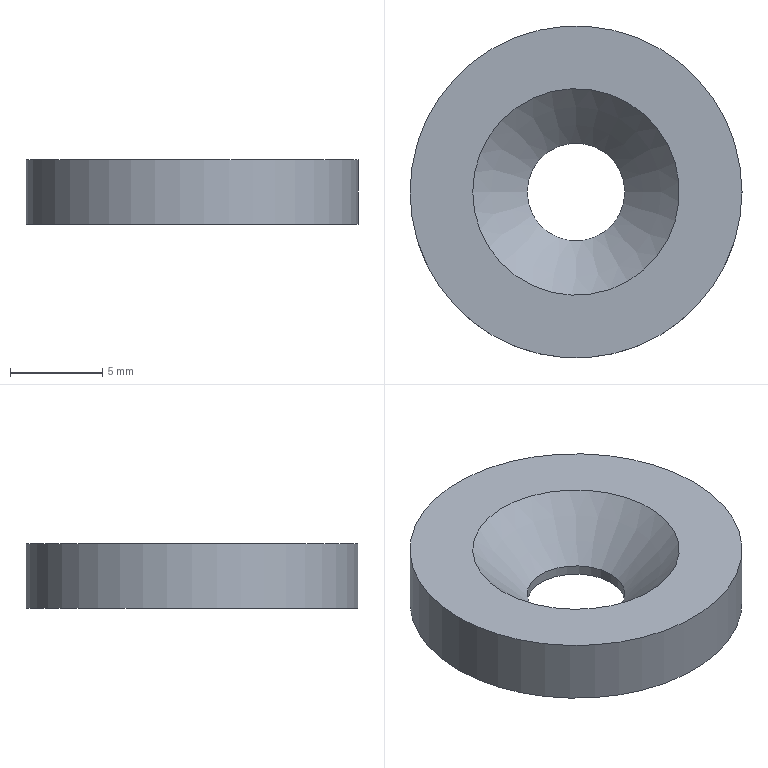Part | NX | 1 solid | 5 faces | box 18 x 18 x 3.5 mm | volume 714.091 mm3 | cylinder 2 | plane 2 | cone 1 | commonest cylinder face diameters 5.3 x1 18 x1
STEP:
#1=CARTESIAN_POINT('',(-2.65,0.,0.55));
#2=VERTEX_POINT('',#1);
#3=CARTESIAN_POINT('',(0.,0.,0.55));
#4=DIRECTION('',(0.,0.,-1.));
#5=DIRECTION('',(-1.,0.,0.));
#6=AXIS2_PLACEMENT_3D('',#3,#4,#5);
#7=CIRCLE('',#6,2.65);
#8=EDGE_CURVE('',#2,#2,#7,.T.);
#9=ORIENTED_EDGE('',*,*,#8,.F.);
#10=EDGE_LOOP('',(#9));
#11=FACE_BOUND('',#10,.T.);
#12=CARTESIAN_POINT('',(-2.65,0.,0.));
#13=VERTEX_POINT('',#12);
#14=CARTESIAN_POINT('',(0.,0.,0.));
#15=DIRECTION('',(0.,0.,-1.));
#16=DIRECTION('',(-1.,0.,0.));
#17=AXIS2_PLACEMENT_3D('',#14,#15,#16);
#18=CIRCLE('',#17,2.65);
#19=EDGE_CURVE('',#13,#13,#18,.T.);
#20=ORIENTED_EDGE('',*,*,#19,.T.);
#21=EDGE_LOOP('',(#20));
#22=FACE_BOUND('',#21,.T.);
#23=CARTESIAN_POINT('',(0.,0.,0.));
#24=DIRECTION('',(0.,0.,-1.));
#25=DIRECTION('',(1.,0.,0.));
#26=AXIS2_PLACEMENT_3D('',#23,#24,#25);
#27=CYLINDRICAL_SURFACE('',#26,2.65);
#28=ADVANCED_FACE('',(#11,#22),#27,.F.);
#29=CARTESIAN_POINT('',(-5.6,0.,3.5));
#30=VERTEX_POINT('',#29);
#31=CARTESIAN_POINT('',(0.,0.,3.5));
#32=DIRECTION('',(0.,0.,-1.));
#33=DIRECTION('',(-1.,0.,0.));
#34=AXIS2_PLACEMENT_3D('',#31,#32,#33);
#35=CIRCLE('',#34,5.6);
#36=EDGE_CURVE('',#30,#30,#35,.T.);
#37=ORIENTED_EDGE('',*,*,#36,.F.);
#38=EDGE_LOOP('',(#37));
#39=FACE_BOUND('',#38,.T.);
#40=ORIENTED_EDGE('',*,*,#8,.T.);
#41=EDGE_LOOP('',(#40));
#42=FACE_BOUND('',#41,.T.);
#43=CARTESIAN_POINT('',(0.,0.,0.55));
#44=DIRECTION('',(0.,0.,1.));
#45=DIRECTION('',(-1.,0.,0.));
#46=AXIS2_PLACEMENT_3D('',#43,#44,#45);
#47=CONICAL_SURFACE('',#46,2.65,45.);
#48=ADVANCED_FACE('',(#39,#42),#47,.F.);
#49=CARTESIAN_POINT('',(-9.,0.,3.5));
#50=VERTEX_POINT('',#49);
#51=CARTESIAN_POINT('',(0.,0.,3.5));
#52=DIRECTION('',(0.,0.,-1.));
#53=DIRECTION('',(-1.,0.,0.));
#54=AXIS2_PLACEMENT_3D('',#51,#52,#53);
#55=CIRCLE('',#54,9.);
#56=EDGE_CURVE('',#50,#50,#55,.T.);
#57=ORIENTED_EDGE('',*,*,#56,.F.);
#58=EDGE_LOOP('',(#57));
#59=FACE_BOUND('',#58,.T.);
#60=ORIENTED_EDGE('',*,*,#36,.T.);
#61=EDGE_LOOP('',(#60));
#62=FACE_BOUND('',#61,.T.);
#63=CARTESIAN_POINT('',(0.,5.6,3.5));
#64=DIRECTION('',(0.,0.,-1.));
#65=DIRECTION('',(1.,0.,0.));
#66=AXIS2_PLACEMENT_3D('',#63,#64,#65);
#67=PLANE('',#66);
#68=ADVANCED_FACE('',(#59,#62),#67,.F.);
#69=CARTESIAN_POINT('',(-9.,0.,0.));
#70=VERTEX_POINT('',#69);
#71=CARTESIAN_POINT('',(0.,0.,0.));
#72=DIRECTION('',(0.,0.,-1.));
#73=DIRECTION('',(-1.,0.,0.));
#74=AXIS2_PLACEMENT_3D('',#71,#72,#73);
#75=CIRCLE('',#74,9.);
#76=EDGE_CURVE('',#70,#70,#75,.T.);
#77=ORIENTED_EDGE('',*,*,#76,.F.);
#78=EDGE_LOOP('',(#77));
#79=FACE_BOUND('',#78,.T.);
#80=ORIENTED_EDGE('',*,*,#56,.T.);
#81=EDGE_LOOP('',(#80));
#82=FACE_BOUND('',#81,.T.);
#83=CARTESIAN_POINT('',(0.,0.,0.));
#84=DIRECTION('',(0.,0.,-1.));
#85=DIRECTION('',(1.,0.,0.));
#86=AXIS2_PLACEMENT_3D('',#83,#84,#85);
#87=CYLINDRICAL_SURFACE('',#86,9.);
#88=ADVANCED_FACE('',(#79,#82),#87,.T.);
#89=ORIENTED_EDGE('',*,*,#19,.F.);
#90=EDGE_LOOP('',(#89));
#91=FACE_BOUND('',#90,.T.);
#92=ORIENTED_EDGE('',*,*,#76,.T.);
#93=EDGE_LOOP('',(#92));
#94=FACE_BOUND('',#93,.T.);
#95=CARTESIAN_POINT('',(0.,9.,0.));
#96=DIRECTION('',(0.,0.,1.));
#97=DIRECTION('',(-1.,0.,0.));
#98=AXIS2_PLACEMENT_3D('',#95,#96,#97);
#99=PLANE('',#98);
#100=ADVANCED_FACE('',(#91,#94),#99,.F.);
#101=CLOSED_SHELL('',(#28,#48,#68,#88,#100));
#102=MANIFOLD_SOLID_BREP('',#101);
#103=(LENGTH_UNIT()NAMED_UNIT(*)SI_UNIT(.MILLI.,.METRE.));
#104=UNCERTAINTY_MEASURE_WITH_UNIT(LENGTH_MEASURE(0.00002),#103,'','');
#105=(NAMED_UNIT(*)PLANE_ANGLE_UNIT()SI_UNIT($,.RADIAN.));
#106=PLANE_ANGLE_MEASURE_WITH_UNIT(PLANE_ANGLE_MEASURE(0.01745),#105);
#107=DIMENSIONAL_EXPONENTS(0.,0.,0.,0.,0.,0.,0.);
#108=(CONVERSION_BASED_UNIT('DEGREE',#106)NAMED_UNIT(#107)PLANE_ANGLE_UNIT());
#109=(NAMED_UNIT(*)SI_UNIT($,.STERADIAN.)SOLID_ANGLE_UNIT());
#110=(GEOMETRIC_REPRESENTATION_CONTEXT(3)GLOBAL_UNCERTAINTY_ASSIGNED_CONTEXT((#104))GLOBAL_UNIT_ASSIGNED_CONTEXT((#103,#108,#109))REPRESENTATION_CONTEXT('',''));
#111=ADVANCED_BREP_SHAPE_REPRESENTATION('',(#102),#110);